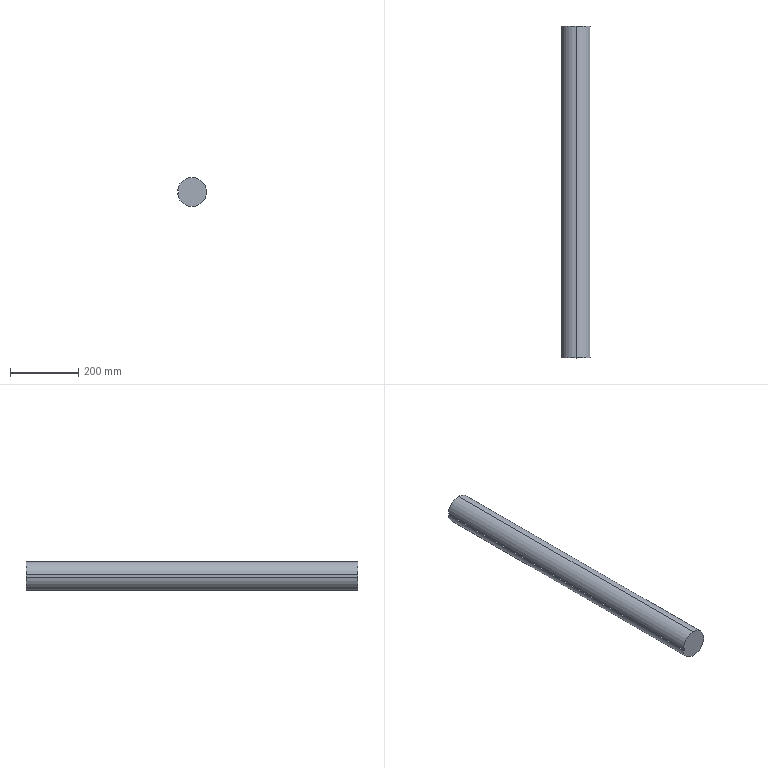Part | STEP file | csb-00002 | 1 solid | 8 faces | box 84.811 x 974 x 85 mm | volume 5496286 mm3 | plane 5 | cylinder 3 | commonest cylinder face diameters 85 x3
STEP:
#1=CARTESIAN_POINT('',(0.,974.,42.5));
#2=VERTEX_POINT('',#1);
#3=CARTESIAN_POINT('',(0.,974.,-42.5));
#4=VERTEX_POINT('',#3);
#5=CARTESIAN_POINT('',(0.,974.,0.));
#6=DIRECTION('',(0.,1.,0.));
#7=DIRECTION('',(0.,0.,1.));
#8=AXIS2_PLACEMENT_3D('',#5,#6,#7);
#9=CIRCLE('',#8,42.5);
#10=EDGE_CURVE('',#2,#4,#9,.T.);
#11=ORIENTED_EDGE('',*,*,#10,.F.);
#12=CARTESIAN_POINT('',(0.,0.,42.5));
#13=VERTEX_POINT('',#12);
#14=CARTESIAN_POINT('',(0.,974.,42.5));
#15=DIRECTION('',(0.,-1.,0.));
#16=VECTOR('',#15,1000.);
#17=LINE('',#14,#16);
#18=EDGE_CURVE('',#2,#13,#17,.T.);
#19=ORIENTED_EDGE('',*,*,#18,.T.);
#20=CARTESIAN_POINT('',(0.,0.,-42.5));
#21=VERTEX_POINT('',#20);
#22=CARTESIAN_POINT('',(0.,0.,0.));
#23=DIRECTION('',(0.,1.,0.));
#24=DIRECTION('',(0.,0.,1.));
#25=AXIS2_PLACEMENT_3D('',#22,#23,#24);
#26=CIRCLE('',#25,42.5);
#27=EDGE_CURVE('',#13,#21,#26,.T.);
#28=ORIENTED_EDGE('',*,*,#27,.T.);
#29=CARTESIAN_POINT('',(0.,974.,-42.5));
#30=DIRECTION('',(0.,-1.,0.));
#31=VECTOR('',#30,1000.);
#32=LINE('',#29,#31);
#33=EDGE_CURVE('',#4,#21,#32,.T.);
#34=ORIENTED_EDGE('',*,*,#33,.F.);
#35=EDGE_LOOP('',(#11,#19,#28,#34));
#36=FACE_OUTER_BOUND('',#35,.T.);
#37=CARTESIAN_POINT('',(0.,974.,0.));
#38=DIRECTION('',(0.,-1.,0.));
#39=DIRECTION('',(0.,0.,-1.));
#40=AXIS2_PLACEMENT_3D('',#37,#38,#39);
#41=CYLINDRICAL_SURFACE('',#40,42.5);
#42=ADVANCED_FACE('',(#36),#41,.T.);
#43=CARTESIAN_POINT('',(-42.311,974.,-4.));
#44=VERTEX_POINT('',#43);
#45=CARTESIAN_POINT('',(0.,974.,0.));
#46=DIRECTION('',(0.,1.,0.));
#47=DIRECTION('',(0.,0.,1.));
#48=AXIS2_PLACEMENT_3D('',#45,#46,#47);
#49=CIRCLE('',#48,42.5);
#50=EDGE_CURVE('',#4,#44,#49,.T.);
#51=ORIENTED_EDGE('',*,*,#50,.F.);
#52=ORIENTED_EDGE('',*,*,#33,.T.);
#53=CARTESIAN_POINT('',(-42.311,0.,-4.));
#54=VERTEX_POINT('',#53);
#55=CARTESIAN_POINT('',(0.,0.,0.));
#56=DIRECTION('',(0.,1.,0.));
#57=DIRECTION('',(0.,0.,1.));
#58=AXIS2_PLACEMENT_3D('',#55,#56,#57);
#59=CIRCLE('',#58,42.5);
#60=EDGE_CURVE('',#21,#54,#59,.T.);
#61=ORIENTED_EDGE('',*,*,#60,.T.);
#62=CARTESIAN_POINT('',(-42.311,974.,-4.));
#63=DIRECTION('',(0.,-1.,0.));
#64=VECTOR('',#63,1000.);
#65=LINE('',#62,#64);
#66=EDGE_CURVE('',#44,#54,#65,.T.);
#67=ORIENTED_EDGE('',*,*,#66,.F.);
#68=EDGE_LOOP('',(#51,#52,#61,#67));
#69=FACE_OUTER_BOUND('',#68,.T.);
#70=CARTESIAN_POINT('',(0.,974.,0.));
#71=DIRECTION('',(0.,-1.,0.));
#72=DIRECTION('',(0.,0.,-1.));
#73=AXIS2_PLACEMENT_3D('',#70,#71,#72);
#74=CYLINDRICAL_SURFACE('',#73,42.5);
#75=ADVANCED_FACE('',(#69),#74,.T.);
#76=ORIENTED_EDGE('',*,*,#18,.F.);
#77=CARTESIAN_POINT('',(-42.311,974.,4.));
#78=VERTEX_POINT('',#77);
#79=CARTESIAN_POINT('',(0.,974.,0.));
#80=DIRECTION('',(0.,1.,0.));
#81=DIRECTION('',(0.,0.,1.));
#82=AXIS2_PLACEMENT_3D('',#79,#80,#81);
#83=CIRCLE('',#82,42.5);
#84=EDGE_CURVE('',#78,#2,#83,.T.);
#85=ORIENTED_EDGE('',*,*,#84,.F.);
#86=CARTESIAN_POINT('',(-42.311,0.,4.));
#87=VERTEX_POINT('',#86);
#88=CARTESIAN_POINT('',(-42.311,974.,4.));
#89=DIRECTION('',(0.,-1.,0.));
#90=VECTOR('',#89,1000.);
#91=LINE('',#88,#90);
#92=EDGE_CURVE('',#78,#87,#91,.T.);
#93=ORIENTED_EDGE('',*,*,#92,.T.);
#94=CARTESIAN_POINT('',(0.,0.,0.));
#95=DIRECTION('',(0.,1.,0.));
#96=DIRECTION('',(0.,0.,1.));
#97=AXIS2_PLACEMENT_3D('',#94,#95,#96);
#98=CIRCLE('',#97,42.5);
#99=EDGE_CURVE('',#87,#13,#98,.T.);
#100=ORIENTED_EDGE('',*,*,#99,.T.);
#101=EDGE_LOOP('',(#76,#85,#93,#100));
#102=FACE_OUTER_BOUND('',#101,.T.);
#103=CARTESIAN_POINT('',(0.,974.,0.));
#104=DIRECTION('',(0.,-1.,0.));
#105=DIRECTION('',(0.,0.,-1.));
#106=AXIS2_PLACEMENT_3D('',#103,#104,#105);
#107=CYLINDRICAL_SURFACE('',#106,42.5);
#108=ADVANCED_FACE('',(#102),#107,.T.);
#109=CARTESIAN_POINT('',(-38.5,0.,-4.));
#110=VERTEX_POINT('',#109);
#111=CARTESIAN_POINT('',(-42.311,0.,-4.));
#112=DIRECTION('',(1.,0.,0.));
#113=VECTOR('',#112,1000.);
#114=LINE('',#111,#113);
#115=EDGE_CURVE('',#54,#110,#114,.T.);
#116=ORIENTED_EDGE('',*,*,#115,.T.);
#117=CARTESIAN_POINT('',(-38.5,974.,-4.));
#118=VERTEX_POINT('',#117);
#119=CARTESIAN_POINT('',(-38.5,974.,-4.));
#120=DIRECTION('',(0.,-1.,0.));
#121=VECTOR('',#120,1000.);
#122=LINE('',#119,#121);
#123=EDGE_CURVE('',#118,#110,#122,.T.);
#124=ORIENTED_EDGE('',*,*,#123,.F.);
#125=CARTESIAN_POINT('',(-42.311,974.,-4.));
#126=DIRECTION('',(1.,0.,0.));
#127=VECTOR('',#126,1000.);
#128=LINE('',#125,#127);
#129=EDGE_CURVE('',#44,#118,#128,.T.);
#130=ORIENTED_EDGE('',*,*,#129,.F.);
#131=ORIENTED_EDGE('',*,*,#66,.T.);
#132=EDGE_LOOP('',(#116,#124,#130,#131));
#133=FACE_OUTER_BOUND('',#132,.T.);
#134=CARTESIAN_POINT('',(-42.311,974.,-4.));
#135=DIRECTION('',(0.,0.,-1.));
#136=DIRECTION('',(-1.,0.,0.));
#137=AXIS2_PLACEMENT_3D('',#134,#135,#136);
#138=PLANE('',#137);
#139=ADVANCED_FACE('',(#133),#138,.F.);
#140=CARTESIAN_POINT('',(-38.5,0.,4.));
#141=VERTEX_POINT('',#140);
#142=CARTESIAN_POINT('',(-38.5,0.,4.));
#143=DIRECTION('',(0.,0.,1.));
#144=VECTOR('',#143,1000.);
#145=LINE('',#142,#144);
#146=EDGE_CURVE('',#110,#141,#145,.T.);
#147=ORIENTED_EDGE('',*,*,#146,.T.);
#148=CARTESIAN_POINT('',(-38.5,974.,4.));
#149=VERTEX_POINT('',#148);
#150=CARTESIAN_POINT('',(-38.5,974.,4.));
#151=DIRECTION('',(0.,-1.,0.));
#152=VECTOR('',#151,1000.);
#153=LINE('',#150,#152);
#154=EDGE_CURVE('',#149,#141,#153,.T.);
#155=ORIENTED_EDGE('',*,*,#154,.F.);
#156=CARTESIAN_POINT('',(-38.5,974.,4.));
#157=DIRECTION('',(0.,0.,1.));
#158=VECTOR('',#157,1000.);
#159=LINE('',#156,#158);
#160=EDGE_CURVE('',#118,#149,#159,.T.);
#161=ORIENTED_EDGE('',*,*,#160,.F.);
#162=ORIENTED_EDGE('',*,*,#123,.T.);
#163=EDGE_LOOP('',(#147,#155,#161,#162));
#164=FACE_OUTER_BOUND('',#163,.T.);
#165=CARTESIAN_POINT('',(-38.5,974.,4.));
#166=DIRECTION('',(1.,0.,0.));
#167=DIRECTION('',(0.,0.,-1.));
#168=AXIS2_PLACEMENT_3D('',#165,#166,#167);
#169=PLANE('',#168);
#170=ADVANCED_FACE('',(#164),#169,.F.);
#171=CARTESIAN_POINT('',(-42.311,0.,4.));
#172=DIRECTION('',(-1.,0.,0.));
#173=VECTOR('',#172,1000.);
#174=LINE('',#171,#173);
#175=EDGE_CURVE('',#141,#87,#174,.T.);
#176=ORIENTED_EDGE('',*,*,#175,.T.);
#177=ORIENTED_EDGE('',*,*,#92,.F.);
#178=CARTESIAN_POINT('',(-42.311,974.,4.));
#179=DIRECTION('',(-1.,0.,0.));
#180=VECTOR('',#179,1000.);
#181=LINE('',#178,#180);
#182=EDGE_CURVE('',#149,#78,#181,.T.);
#183=ORIENTED_EDGE('',*,*,#182,.F.);
#184=ORIENTED_EDGE('',*,*,#154,.T.);
#185=EDGE_LOOP('',(#176,#177,#183,#184));
#186=FACE_OUTER_BOUND('',#185,.T.);
#187=CARTESIAN_POINT('',(-42.311,974.,4.));
#188=DIRECTION('',(0.,0.,1.));
#189=DIRECTION('',(1.,0.,0.));
#190=AXIS2_PLACEMENT_3D('',#187,#188,#189);
#191=PLANE('',#190);
#192=ADVANCED_FACE('',(#186),#191,.F.);
#193=ORIENTED_EDGE('',*,*,#84,.T.);
#194=ORIENTED_EDGE('',*,*,#10,.T.);
#195=ORIENTED_EDGE('',*,*,#50,.T.);
#196=ORIENTED_EDGE('',*,*,#129,.T.);
#197=ORIENTED_EDGE('',*,*,#160,.T.);
#198=ORIENTED_EDGE('',*,*,#182,.T.);
#199=EDGE_LOOP('',(#193,#194,#195,#196,#197,#198));
#200=FACE_OUTER_BOUND('',#199,.T.);
#201=CARTESIAN_POINT('',(0.,974.,0.));
#202=DIRECTION('',(0.,1.,0.));
#203=DIRECTION('',(0.,0.,1.));
#204=AXIS2_PLACEMENT_3D('',#201,#202,#203);
#205=PLANE('',#204);
#206=ADVANCED_FACE('',(#200),#205,.T.);
#207=ORIENTED_EDGE('',*,*,#99,.F.);
#208=ORIENTED_EDGE('',*,*,#175,.F.);
#209=ORIENTED_EDGE('',*,*,#146,.F.);
#210=ORIENTED_EDGE('',*,*,#115,.F.);
#211=ORIENTED_EDGE('',*,*,#60,.F.);
#212=ORIENTED_EDGE('',*,*,#27,.F.);
#213=EDGE_LOOP('',(#207,#208,#209,#210,#211,#212));
#214=FACE_OUTER_BOUND('',#213,.T.);
#215=CARTESIAN_POINT('',(0.,0.,0.));
#216=DIRECTION('',(0.,1.,0.));
#217=DIRECTION('',(0.,0.,1.));
#218=AXIS2_PLACEMENT_3D('',#215,#216,#217);
#219=PLANE('',#218);
#220=ADVANCED_FACE('',(#214),#219,.F.);
#221=CLOSED_SHELL('',(#42,#75,#108,#139,#170,#192,#206,#220));
#222=MANIFOLD_SOLID_BREP('',#221);
#223=CARTESIAN_POINT('',(0.,0.,0.));
#224=DIRECTION('',(0.,0.,1.));
#225=DIRECTION('',(1.,0.,0.));
#226=AXIS2_PLACEMENT_3D('',#223,#224,#225);
#227=(LENGTH_UNIT()NAMED_UNIT(*)SI_UNIT(.MILLI.,.METRE.));
#228=UNCERTAINTY_MEASURE_WITH_UNIT(LENGTH_MEASURE(0.00001),#227,'','');
#229=(NAMED_UNIT(*)PLANE_ANGLE_UNIT()SI_UNIT($,.RADIAN.));
#230=(NAMED_UNIT(*)SI_UNIT($,.STERADIAN.)SOLID_ANGLE_UNIT());
#231=(GEOMETRIC_REPRESENTATION_CONTEXT(3)GLOBAL_UNCERTAINTY_ASSIGNED_CONTEXT((#228))GLOBAL_UNIT_ASSIGNED_CONTEXT((#227,#229,#230))REPRESENTATION_CONTEXT('',''));
#232=ADVANCED_BREP_SHAPE_REPRESENTATION('',(#222,#226),#231);